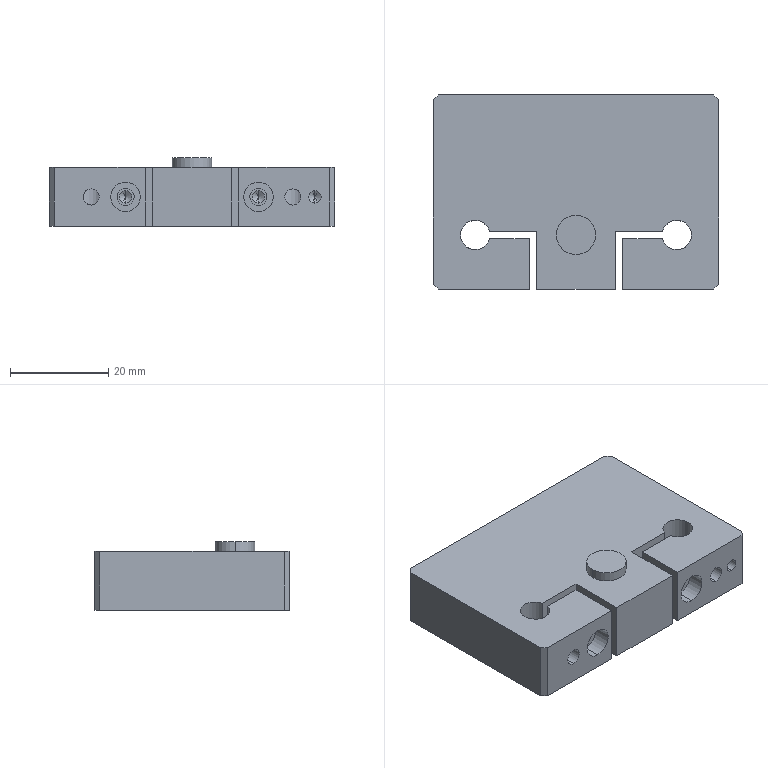Part | SolidWorks | features HoleWzd 4, ICE 2, Chamfer 1, Extrusion 1, MirrorPattern 1 | 2 solids | 64 faces | box 58 x 39.5 x 14 mm | volume 25416 mm3 | cylinder 29 | plane 25 | cone 10 | commonest cylinder face diameters 3.3 x8 6 x7 2.5 x6 3.5 x4 8 x4